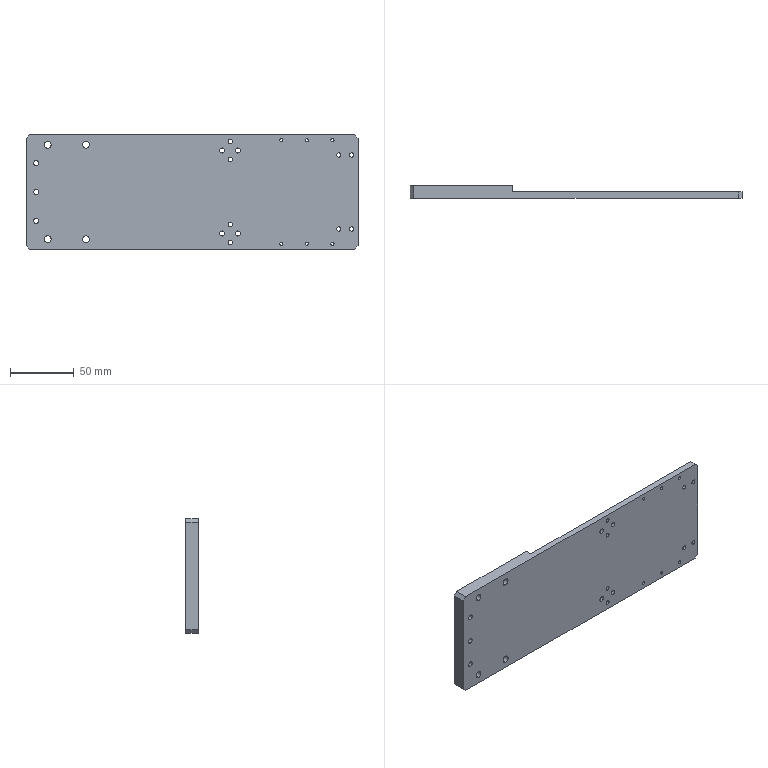Part | SolidWorks | features HoleWzd 7, Chamfer 1, Extrusion 1, ICE 1 | 1 solid | 74 faces | box 260 x 10 x 90 mm | volume 149509 mm3 | cylinder 58 | plane 16 | commonest cylinder face diameters 3.3 x16 2.5 x12 4 x8 5.5 x8 10 x8 4.2 x6